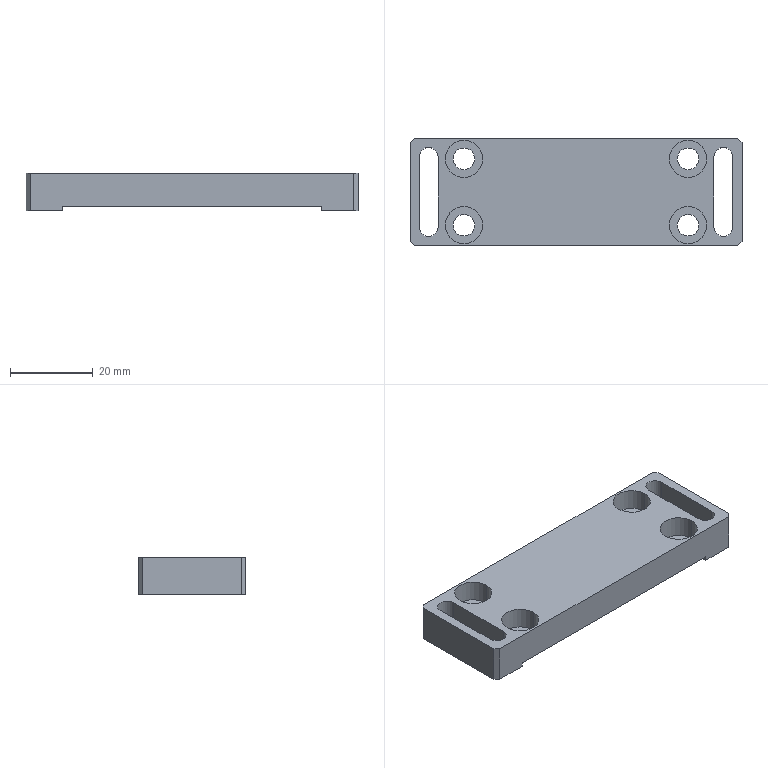Part | SolidWorks | features ICE 4, Chamfer 1, Extrusion 1, MirrorPattern 1 | 1 solid | 42 faces | box 80 x 26 x 9 mm | volume 13853 mm3 | plane 22 | cylinder 20 | commonest cylinder face diameters 5.2 x8 9 x8 4.5 x4
STEP:
#1=CARTESIAN_POINT('',(22.5,-8.,3.8));
#2=VERTEX_POINT('',#1);
#3=CARTESIAN_POINT('',(31.5,-8.,3.8));
#4=VERTEX_POINT('',#3);
#5=CARTESIAN_POINT('',(27.,-8.,3.8));
#6=DIRECTION('',(0.,0.,1.));
#7=DIRECTION('',(1.,0.,0.));
#8=AXIS2_PLACEMENT_3D('',#5,#6,#7);
#9=CIRCLE('',#8,4.5);
#10=EDGE_CURVE('',#2,#4,#9,.T.);
#11=ORIENTED_EDGE('',*,*,#10,.F.);
#12=CARTESIAN_POINT('',(22.5,-8.,9.));
#13=VERTEX_POINT('',#12);
#14=CARTESIAN_POINT('',(22.5,-8.,3.8));
#15=DIRECTION('',(0.,0.,1.));
#16=VECTOR('',#15,1000.);
#17=LINE('',#14,#16);
#18=EDGE_CURVE('',#2,#13,#17,.T.);
#19=ORIENTED_EDGE('',*,*,#18,.T.);
#20=CARTESIAN_POINT('',(31.5,-8.,9.));
#21=VERTEX_POINT('',#20);
#22=CARTESIAN_POINT('',(27.,-8.,9.));
#23=DIRECTION('',(0.,0.,1.));
#24=DIRECTION('',(1.,0.,0.));
#25=AXIS2_PLACEMENT_3D('',#22,#23,#24);
#26=CIRCLE('',#25,4.5);
#27=EDGE_CURVE('',#13,#21,#26,.T.);
#28=ORIENTED_EDGE('',*,*,#27,.T.);
#29=CARTESIAN_POINT('',(31.5,-8.,3.8));
#30=DIRECTION('',(0.,0.,1.));
#31=VECTOR('',#30,1000.);
#32=LINE('',#29,#31);
#33=EDGE_CURVE('',#4,#21,#32,.T.);
#34=ORIENTED_EDGE('',*,*,#33,.F.);
#35=EDGE_LOOP('',(#11,#19,#28,#34));
#36=FACE_OUTER_BOUND('',#35,.T.);
#37=CARTESIAN_POINT('',(27.,-8.,3.8));
#38=DIRECTION('',(0.,0.,1.));
#39=DIRECTION('',(1.,0.,0.));
#40=AXIS2_PLACEMENT_3D('',#37,#38,#39);
#41=CYLINDRICAL_SURFACE('',#40,4.5);
#42=ADVANCED_FACE('',(#36),#41,.F.);
#43=CARTESIAN_POINT('',(22.5,8.,3.8));
#44=VERTEX_POINT('',#43);
#45=CARTESIAN_POINT('',(31.5,8.,3.8));
#46=VERTEX_POINT('',#45);
#47=CARTESIAN_POINT('',(27.,8.,3.8));
#48=DIRECTION('',(0.,0.,1.));
#49=DIRECTION('',(1.,0.,0.));
#50=AXIS2_PLACEMENT_3D('',#47,#48,#49);
#51=CIRCLE('',#50,4.5);
#52=EDGE_CURVE('',#44,#46,#51,.T.);
#53=ORIENTED_EDGE('',*,*,#52,.F.);
#54=CARTESIAN_POINT('',(22.5,8.,9.));
#55=VERTEX_POINT('',#54);
#56=CARTESIAN_POINT('',(22.5,8.,3.8));
#57=DIRECTION('',(0.,0.,1.));
#58=VECTOR('',#57,1000.);
#59=LINE('',#56,#58);
#60=EDGE_CURVE('',#44,#55,#59,.T.);
#61=ORIENTED_EDGE('',*,*,#60,.T.);
#62=CARTESIAN_POINT('',(31.5,8.,9.));
#63=VERTEX_POINT('',#62);
#64=CARTESIAN_POINT('',(27.,8.,9.));
#65=DIRECTION('',(0.,0.,1.));
#66=DIRECTION('',(1.,0.,0.));
#67=AXIS2_PLACEMENT_3D('',#64,#65,#66);
#68=CIRCLE('',#67,4.5);
#69=EDGE_CURVE('',#55,#63,#68,.T.);
#70=ORIENTED_EDGE('',*,*,#69,.T.);
#71=CARTESIAN_POINT('',(31.5,8.,3.8));
#72=DIRECTION('',(0.,0.,1.));
#73=VECTOR('',#72,1000.);
#74=LINE('',#71,#73);
#75=EDGE_CURVE('',#46,#63,#74,.T.);
#76=ORIENTED_EDGE('',*,*,#75,.F.);
#77=EDGE_LOOP('',(#53,#61,#70,#76));
#78=FACE_OUTER_BOUND('',#77,.T.);
#79=CARTESIAN_POINT('',(27.,8.,3.8));
#80=DIRECTION('',(0.,0.,1.));
#81=DIRECTION('',(1.,0.,0.));
#82=AXIS2_PLACEMENT_3D('',#79,#80,#81);
#83=CYLINDRICAL_SURFACE('',#82,4.5);
#84=ADVANCED_FACE('',(#78),#83,.F.);
#85=CARTESIAN_POINT('',(-31.5,8.,3.8));
#86=VERTEX_POINT('',#85);
#87=CARTESIAN_POINT('',(-22.5,8.,3.8));
#88=VERTEX_POINT('',#87);
#89=CARTESIAN_POINT('',(-27.,8.,3.8));
#90=DIRECTION('',(0.,0.,1.));
#91=DIRECTION('',(1.,0.,0.));
#92=AXIS2_PLACEMENT_3D('',#89,#90,#91);
#93=CIRCLE('',#92,4.5);
#94=EDGE_CURVE('',#86,#88,#93,.T.);
#95=ORIENTED_EDGE('',*,*,#94,.F.);
#96=CARTESIAN_POINT('',(-31.5,8.,9.));
#97=VERTEX_POINT('',#96);
#98=CARTESIAN_POINT('',(-31.5,8.,3.8));
#99=DIRECTION('',(0.,0.,1.));
#100=VECTOR('',#99,1000.);
#101=LINE('',#98,#100);
#102=EDGE_CURVE('',#86,#97,#101,.T.);
#103=ORIENTED_EDGE('',*,*,#102,.T.);
#104=CARTESIAN_POINT('',(-22.5,8.,9.));
#105=VERTEX_POINT('',#104);
#106=CARTESIAN_POINT('',(-27.,8.,9.));
#107=DIRECTION('',(0.,0.,1.));
#108=DIRECTION('',(1.,0.,0.));
#109=AXIS2_PLACEMENT_3D('',#106,#107,#108);
#110=CIRCLE('',#109,4.5);
#111=EDGE_CURVE('',#97,#105,#110,.T.);
#112=ORIENTED_EDGE('',*,*,#111,.T.);
#113=CARTESIAN_POINT('',(-22.5,8.,3.8));
#114=DIRECTION('',(0.,0.,1.));
#115=VECTOR('',#114,1000.);
#116=LINE('',#113,#115);
#117=EDGE_CURVE('',#88,#105,#116,.T.);
#118=ORIENTED_EDGE('',*,*,#117,.F.);
#119=EDGE_LOOP('',(#95,#103,#112,#118));
#120=FACE_OUTER_BOUND('',#119,.T.);
#121=CARTESIAN_POINT('',(-27.,8.,3.8));
#122=DIRECTION('',(0.,0.,1.));
#123=DIRECTION('',(1.,0.,0.));
#124=AXIS2_PLACEMENT_3D('',#121,#122,#123);
#125=CYLINDRICAL_SURFACE('',#124,4.5);
#126=ADVANCED_FACE('',(#120),#125,.F.);
#127=CARTESIAN_POINT('',(-31.5,-8.,3.8));
#128=VERTEX_POINT('',#127);
#129=CARTESIAN_POINT('',(-22.5,-8.,3.8));
#130=VERTEX_POINT('',#129);
#131=CARTESIAN_POINT('',(-27.,-8.,3.8));
#132=DIRECTION('',(0.,0.,1.));
#133=DIRECTION('',(1.,0.,0.));
#134=AXIS2_PLACEMENT_3D('',#131,#132,#133);
#135=CIRCLE('',#134,4.5);
#136=EDGE_CURVE('',#128,#130,#135,.T.);
#137=ORIENTED_EDGE('',*,*,#136,.F.);
#138=CARTESIAN_POINT('',(-31.5,-8.,9.));
#139=VERTEX_POINT('',#138);
#140=CARTESIAN_POINT('',(-31.5,-8.,3.8));
#141=DIRECTION('',(0.,0.,1.));
#142=VECTOR('',#141,1000.);
#143=LINE('',#140,#142);
#144=EDGE_CURVE('',#128,#139,#143,.T.);
#145=ORIENTED_EDGE('',*,*,#144,.T.);
#146=CARTESIAN_POINT('',(-22.5,-8.,9.));
#147=VERTEX_POINT('',#146);
#148=CARTESIAN_POINT('',(-27.,-8.,9.));
#149=DIRECTION('',(0.,0.,1.));
#150=DIRECTION('',(1.,0.,0.));
#151=AXIS2_PLACEMENT_3D('',#148,#149,#150);
#152=CIRCLE('',#151,4.5);
#153=EDGE_CURVE('',#139,#147,#152,.T.);
#154=ORIENTED_EDGE('',*,*,#153,.T.);
#155=CARTESIAN_POINT('',(-22.5,-8.,3.8));
#156=DIRECTION('',(0.,0.,1.));
#157=VECTOR('',#156,1000.);
#158=LINE('',#155,#157);
#159=EDGE_CURVE('',#130,#147,#158,.T.);
#160=ORIENTED_EDGE('',*,*,#159,.F.);
#161=EDGE_LOOP('',(#137,#145,#154,#160));
#162=FACE_OUTER_BOUND('',#161,.T.);
#163=CARTESIAN_POINT('',(-27.,-8.,3.8));
#164=DIRECTION('',(0.,0.,1.));
#165=DIRECTION('',(1.,0.,0.));
#166=AXIS2_PLACEMENT_3D('',#163,#164,#165);
#167=CYLINDRICAL_SURFACE('',#166,4.5);
#168=ADVANCED_FACE('',(#162),#167,.F.);
#169=CARTESIAN_POINT('',(-29.6,-8.,1.));
#170=VERTEX_POINT('',#169);
#171=CARTESIAN_POINT('',(-24.4,-8.,1.));
#172=VERTEX_POINT('',#171);
#173=CARTESIAN_POINT('',(-27.,-8.,1.));
#174=DIRECTION('',(0.,0.,1.));
#175=DIRECTION('',(-1.,0.,0.));
#176=AXIS2_PLACEMENT_3D('',#173,#174,#175);
#177=CIRCLE('',#176,2.6);
#178=EDGE_CURVE('',#170,#172,#177,.T.);
#179=ORIENTED_EDGE('',*,*,#178,.F.);
#180=CARTESIAN_POINT('',(-29.6,-8.,3.8));
#181=VERTEX_POINT('',#180);
#182=CARTESIAN_POINT('',(-29.6,-8.,-0.001));
#183=DIRECTION('',(0.,0.,1.));
#184=VECTOR('',#183,1000.);
#185=LINE('',#182,#184);
#186=EDGE_CURVE('',#170,#181,#185,.T.);
#187=ORIENTED_EDGE('',*,*,#186,.T.);
#188=CARTESIAN_POINT('',(-24.4,-8.,3.8));
#189=VERTEX_POINT('',#188);
#190=CARTESIAN_POINT('',(-27.,-8.,3.8));
#191=DIRECTION('',(0.,0.,-1.));
#192=DIRECTION('',(1.,0.,0.));
#193=AXIS2_PLACEMENT_3D('',#190,#191,#192);
#194=CIRCLE('',#193,2.6);
#195=EDGE_CURVE('',#189,#181,#194,.T.);
#196=ORIENTED_EDGE('',*,*,#195,.F.);
#197=CARTESIAN_POINT('',(-24.4,-8.,-0.001));
#198=DIRECTION('',(0.,0.,1.));
#199=VECTOR('',#198,1000.);
#200=LINE('',#197,#199);
#201=EDGE_CURVE('',#172,#189,#200,.T.);
#202=ORIENTED_EDGE('',*,*,#201,.F.);
#203=EDGE_LOOP('',(#179,#187,#196,#202));
#204=FACE_OUTER_BOUND('',#203,.T.);
#205=CARTESIAN_POINT('',(-27.,-8.,-0.001));
#206=DIRECTION('',(0.,0.,1.));
#207=DIRECTION('',(1.,0.,0.));
#208=AXIS2_PLACEMENT_3D('',#205,#206,#207);
#209=CYLINDRICAL_SURFACE('',#208,2.6);
#210=ADVANCED_FACE('',(#204),#209,.F.);
#211=CARTESIAN_POINT('',(-29.6,8.,1.));
#212=VERTEX_POINT('',#211);
#213=CARTESIAN_POINT('',(-24.4,8.,1.));
#214=VERTEX_POINT('',#213);
#215=CARTESIAN_POINT('',(-27.,8.,1.));
#216=DIRECTION('',(0.,0.,1.));
#217=DIRECTION('',(-1.,0.,0.));
#218=AXIS2_PLACEMENT_3D('',#215,#216,#217);
#219=CIRCLE('',#218,2.6);
#220=EDGE_CURVE('',#212,#214,#219,.T.);
#221=ORIENTED_EDGE('',*,*,#220,.F.);
#222=CARTESIAN_POINT('',(-29.6,8.,3.8));
#223=VERTEX_POINT('',#222);
#224=CARTESIAN_POINT('',(-29.6,8.,-0.001));
#225=DIRECTION('',(0.,0.,1.));
#226=VECTOR('',#225,1000.);
#227=LINE('',#224,#226);
#228=EDGE_CURVE('',#212,#223,#227,.T.);
#229=ORIENTED_EDGE('',*,*,#228,.T.);
#230=CARTESIAN_POINT('',(-24.4,8.,3.8));
#231=VERTEX_POINT('',#230);
#232=CARTESIAN_POINT('',(-27.,8.,3.8));
#233=DIRECTION('',(0.,0.,-1.));
#234=DIRECTION('',(1.,0.,0.));
#235=AXIS2_PLACEMENT_3D('',#232,#233,#234);
#236=CIRCLE('',#235,2.6);
#237=EDGE_CURVE('',#231,#223,#236,.T.);
#238=ORIENTED_EDGE('',*,*,#237,.F.);
#239=CARTESIAN_POINT('',(-24.4,8.,-0.001));
#240=DIRECTION('',(0.,0.,1.));
#241=VECTOR('',#240,1000.);
#242=LINE('',#239,#241);
#243=EDGE_CURVE('',#214,#231,#242,.T.);
#244=ORIENTED_EDGE('',*,*,#243,.F.);
#245=EDGE_LOOP('',(#221,#229,#238,#244));
#246=FACE_OUTER_BOUND('',#245,.T.);
#247=CARTESIAN_POINT('',(-27.,8.,-0.001));
#248=DIRECTION('',(0.,0.,1.));
#249=DIRECTION('',(1.,0.,0.));
#250=AXIS2_PLACEMENT_3D('',#247,#248,#249);
#251=CYLINDRICAL_SURFACE('',#250,2.6);
#252=ADVANCED_FACE('',(#246),#251,.F.);
#253=CARTESIAN_POINT('',(24.4,8.,1.));
#254=VERTEX_POINT('',#253);
#255=CARTESIAN_POINT('',(29.6,8.,1.));
#256=VERTEX_POINT('',#255);
#257=CARTESIAN_POINT('',(27.,8.,1.));
#258=DIRECTION('',(0.,0.,1.));
#259=DIRECTION('',(-1.,0.,0.));
#260=AXIS2_PLACEMENT_3D('',#257,#258,#259);
#261=CIRCLE('',#260,2.6);
#262=EDGE_CURVE('',#254,#256,#261,.T.);
#263=ORIENTED_EDGE('',*,*,#262,.F.);
#264=CARTESIAN_POINT('',(24.4,8.,3.8));
#265=VERTEX_POINT('',#264);
#266=CARTESIAN_POINT('',(24.4,8.,-0.001));
#267=DIRECTION('',(0.,0.,1.));
#268=VECTOR('',#267,1000.);
#269=LINE('',#266,#268);
#270=EDGE_CURVE('',#254,#265,#269,.T.);
#271=ORIENTED_EDGE('',*,*,#270,.T.);
#272=CARTESIAN_POINT('',(29.6,8.,3.8));
#273=VERTEX_POINT('',#272);
#274=CARTESIAN_POINT('',(27.,8.,3.8));
#275=DIRECTION('',(0.,0.,-1.));
#276=DIRECTION('',(1.,0.,0.));
#277=AXIS2_PLACEMENT_3D('',#274,#275,#276);
#278=CIRCLE('',#277,2.6);
#279=EDGE_CURVE('',#273,#265,#278,.T.);
#280=ORIENTED_EDGE('',*,*,#279,.F.);
#281=CARTESIAN_POINT('',(29.6,8.,-0.001));
#282=DIRECTION('',(0.,0.,1.));
#283=VECTOR('',#282,1000.);
#284=LINE('',#281,#283);
#285=EDGE_CURVE('',#256,#273,#284,.T.);
#286=ORIENTED_EDGE('',*,*,#285,.F.);
#287=EDGE_LOOP('',(#263,#271,#280,#286));
#288=FACE_OUTER_BOUND('',#287,.T.);
#289=CARTESIAN_POINT('',(27.,8.,-0.001));
#290=DIRECTION('',(0.,0.,1.));
#291=DIRECTION('',(1.,0.,0.));
#292=AXIS2_PLACEMENT_3D('',#289,#290,#291);
#293=CYLINDRICAL_SURFACE('',#292,2.6);
#294=ADVANCED_FACE('',(#288),#293,.F.);
#295=CARTESIAN_POINT('',(24.4,-8.,1.));
#296=VERTEX_POINT('',#295);
#297=CARTESIAN_POINT('',(29.6,-8.,1.));
#298=VERTEX_POINT('',#297);
#299=CARTESIAN_POINT('',(27.,-8.,1.));
#300=DIRECTION('',(0.,0.,1.));
#301=DIRECTION('',(-1.,0.,0.));
#302=AXIS2_PLACEMENT_3D('',#299,#300,#301);
#303=CIRCLE('',#302,2.6);
#304=EDGE_CURVE('',#296,#298,#303,.T.);
#305=ORIENTED_EDGE('',*,*,#304,.F.);
#306=CARTESIAN_POINT('',(24.4,-8.,3.8));
#307=VERTEX_POINT('',#306);
#308=CARTESIAN_POINT('',(24.4,-8.,-0.001));
#309=DIRECTION('',(0.,0.,1.));
#310=VECTOR('',#309,1000.);
#311=LINE('',#308,#310);
#312=EDGE_CURVE('',#296,#307,#311,.T.);
#313=ORIENTED_EDGE('',*,*,#312,.T.);
#314=CARTESIAN_POINT('',(29.6,-8.,3.8));
#315=VERTEX_POINT('',#314);
#316=CARTESIAN_POINT('',(27.,-8.,3.8));
#317=DIRECTION('',(0.,0.,-1.));
#318=DIRECTION('',(1.,0.,0.));
#319=AXIS2_PLACEMENT_3D('',#316,#317,#318);
#320=CIRCLE('',#319,2.6);
#321=EDGE_CURVE('',#315,#307,#320,.T.);
#322=ORIENTED_EDGE('',*,*,#321,.F.);
#323=CARTESIAN_POINT('',(29.6,-8.,-0.001));
#324=DIRECTION('',(0.,0.,1.));
#325=VECTOR('',#324,1000.);
#326=LINE('',#323,#325);
#327=EDGE_CURVE('',#298,#315,#326,.T.);
#328=ORIENTED_EDGE('',*,*,#327,.F.);
#329=EDGE_LOOP('',(#305,#313,#322,#328));
#330=FACE_OUTER_BOUND('',#329,.T.);
#331=CARTESIAN_POINT('',(27.,-8.,-0.001));
#332=DIRECTION('',(0.,0.,1.));
#333=DIRECTION('',(1.,0.,0.));
#334=AXIS2_PLACEMENT_3D('',#331,#332,#333);
#335=CYLINDRICAL_SURFACE('',#334,2.6);
#336=ADVANCED_FACE('',(#330),#335,.F.);
#337=CARTESIAN_POINT('',(-33.25,8.5,0.));
#338=VERTEX_POINT('',#337);
#339=CARTESIAN_POINT('',(-37.75,8.5,0.));
#340=VERTEX_POINT('',#339);
#341=CARTESIAN_POINT('',(-35.5,8.5,0.));
#342=DIRECTION('',(0.,0.,1.));
#343=DIRECTION('',(1.,0.,0.));
#344=AXIS2_PLACEMENT_3D('',#341,#342,#343);
#345=CIRCLE('',#344,2.25);
#346=EDGE_CURVE('',#338,#340,#345,.T.);
#347=ORIENTED_EDGE('',*,*,#346,.T.);
#348=CARTESIAN_POINT('',(-37.75,-8.5,0.));
#349=VERTEX_POINT('',#348);
#350=CARTESIAN_POINT('',(-37.75,8.5,0.));
#351=DIRECTION('',(0.,-1.,0.));
#352=VECTOR('',#351,1000.);
#353=LINE('',#350,#352);
#354=EDGE_CURVE('',#340,#349,#353,.T.);
#355=ORIENTED_EDGE('',*,*,#354,.T.);
#356=CARTESIAN_POINT('',(-33.25,-8.5,0.));
#357=VERTEX_POINT('',#356);
#358=CARTESIAN_POINT('',(-35.5,-8.5,0.));
#359=DIRECTION('',(0.,0.,1.));
#360=DIRECTION('',(1.,0.,0.));
#361=AXIS2_PLACEMENT_3D('',#358,#359,#360);
#362=CIRCLE('',#361,2.25);
#363=EDGE_CURVE('',#349,#357,#362,.T.);
#364=ORIENTED_EDGE('',*,*,#363,.T.);
#365=CARTESIAN_POINT('',(-33.25,8.5,0.));
#366=DIRECTION('',(0.,1.,0.));
#367=VECTOR('',#366,1000.);
#368=LINE('',#365,#367);
#369=EDGE_CURVE('',#357,#338,#368,.T.);
#370=ORIENTED_EDGE('',*,*,#369,.T.);
#371=EDGE_LOOP('',(#347,#355,#364,#370));
#372=FACE_BOUND('',#371,.T.);
#373=CARTESIAN_POINT('',(-39.,-13.,0.));
#374=VERTEX_POINT('',#373);
#375=CARTESIAN_POINT('',(-31.25,-13.,0.));
#376=VERTEX_POINT('',#375);
#377=CARTESIAN_POINT('',(-40.,-13.,0.));
#378=DIRECTION('',(1.,0.,0.));
#379=VECTOR('',#378,1000.);
#380=LINE('',#377,#379);
#381=EDGE_CURVE('',#374,#376,#380,.T.);
#382=ORIENTED_EDGE('',*,*,#381,.F.);
#383=CARTESIAN_POINT('',(-40.,-12.,0.));
#384=VERTEX_POINT('',#383);
#385=CARTESIAN_POINT('',(-39.,-13.,0.));
#386=DIRECTION('',(-0.7071,0.7071,0.));
#387=VECTOR('',#386,1000.);
#388=LINE('',#385,#387);
#389=EDGE_CURVE('',#374,#384,#388,.T.);
#390=ORIENTED_EDGE('',*,*,#389,.T.);
#391=CARTESIAN_POINT('',(-40.,12.,0.));
#392=VERTEX_POINT('',#391);
#393=CARTESIAN_POINT('',(-40.,13.,0.));
#394=DIRECTION('',(0.,-1.,0.));
#395=VECTOR('',#394,1000.);
#396=LINE('',#393,#395);
#397=EDGE_CURVE('',#392,#384,#396,.T.);
#398=ORIENTED_EDGE('',*,*,#397,.F.);
#399=CARTESIAN_POINT('',(-39.,13.,0.));
#400=VERTEX_POINT('',#399);
#401=CARTESIAN_POINT('',(-40.,12.,0.));
#402=DIRECTION('',(0.7071,0.7071,0.));
#403=VECTOR('',#402,1000.);
#404=LINE('',#401,#403);
#405=EDGE_CURVE('',#392,#400,#404,.T.);
#406=ORIENTED_EDGE('',*,*,#405,.T.);
#407=CARTESIAN_POINT('',(-31.25,13.,0.));
#408=VERTEX_POINT('',#407);
#409=CARTESIAN_POINT('',(-40.,13.,0.));
#410=DIRECTION('',(-1.,0.,0.));
#411=VECTOR('',#410,1000.);
#412=LINE('',#409,#411);
#413=EDGE_CURVE('',#408,#400,#412,.T.);
#414=ORIENTED_EDGE('',*,*,#413,.F.);
#415=CARTESIAN_POINT('',(-31.25,13.,0.));
#416=DIRECTION('',(0.,1.,0.));
#417=VECTOR('',#416,1000.);
#418=LINE('',#415,#417);
#419=EDGE_CURVE('',#376,#408,#418,.T.);
#420=ORIENTED_EDGE('',*,*,#419,.F.);
#421=EDGE_LOOP('',(#382,#390,#398,#406,#414,#420));
#422=FACE_OUTER_BOUND('',#421,.T.);
#423=CARTESIAN_POINT('',(40.,-13.,0.));
#424=DIRECTION('',(0.,0.,1.));
#425=DIRECTION('',(1.,0.,0.));
#426=AXIS2_PLACEMENT_3D('',#423,#424,#425);
#427=PLANE('',#426);
#428=ADVANCED_FACE('',(#372,#422),#427,.F.);
#429=ORIENTED_EDGE('',*,*,#312,.F.);
#430=CARTESIAN_POINT('',(27.,-8.,1.));
#431=DIRECTION('',(0.,0.,1.));
#432=DIRECTION('',(-1.,0.,0.));
#433=AXIS2_PLACEMENT_3D('',#430,#431,#432);
#434=CIRCLE('',#433,2.6);
#435=EDGE_CURVE('',#298,#296,#434,.T.);
#436=ORIENTED_EDGE('',*,*,#435,.F.);
#437=ORIENTED_EDGE('',*,*,#327,.T.);
#438=CARTESIAN_POINT('',(27.,-8.,3.8));
#439=DIRECTION('',(0.,0.,-1.));
#440=DIRECTION('',(1.,0.,0.));
#441=AXIS2_PLACEMENT_3D('',#438,#439,#440);
#442=CIRCLE('',#441,2.6);
#443=EDGE_CURVE('',#307,#315,#442,.T.);
#444=ORIENTED_EDGE('',*,*,#443,.F.);
#445=EDGE_LOOP('',(#429,#436,#437,#444));
#446=FACE_OUTER_BOUND('',#445,.T.);
#447=CARTESIAN_POINT('',(27.,-8.,-0.001));
#448=DIRECTION('',(0.,0.,1.));
#449=DIRECTION('',(1.,0.,0.));
#450=AXIS2_PLACEMENT_3D('',#447,#448,#449);
#451=CYLINDRICAL_SURFACE('',#450,2.6);
#452=ADVANCED_FACE('',(#446),#451,.F.);
#453=ORIENTED_EDGE('',*,*,#270,.F.);
#454=CARTESIAN_POINT('',(27.,8.,1.));
#455=DIRECTION('',(0.,0.,1.));
#456=DIRECTION('',(-1.,0.,0.));
#457=AXIS2_PLACEMENT_3D('',#454,#455,#456);
#458=CIRCLE('',#457,2.6);
#459=EDGE_CURVE('',#256,#254,#458,.T.);
#460=ORIENTED_EDGE('',*,*,#459,.F.);
#461=ORIENTED_EDGE('',*,*,#285,.T.);
#462=CARTESIAN_POINT('',(27.,8.,3.8));
#463=DIRECTION('',(0.,0.,-1.));
#464=DIRECTION('',(1.,0.,0.));
#465=AXIS2_PLACEMENT_3D('',#462,#463,#464);
#466=CIRCLE('',#465,2.6);
#467=EDGE_CURVE('',#265,#273,#466,.T.);
#468=ORIENTED_EDGE('',*,*,#467,.F.);
#469=EDGE_LOOP('',(#453,#460,#461,#468));
#470=FACE_OUTER_BOUND('',#469,.T.);
#471=CARTESIAN_POINT('',(27.,8.,-0.001));
#472=DIRECTION('',(0.,0.,1.));
#473=DIRECTION('',(1.,0.,0.));
#474=AXIS2_PLACEMENT_3D('',#471,#472,#473);
#475=CYLINDRICAL_SURFACE('',#474,2.6);
#476=ADVANCED_FACE('',(#470),#475,.F.);
#477=ORIENTED_EDGE('',*,*,#228,.F.);
#478=CARTESIAN_POINT('',(-27.,8.,1.));
#479=DIRECTION('',(0.,0.,1.));
#480=DIRECTION('',(-1.,0.,0.));
#481=AXIS2_PLACEMENT_3D('',#478,#479,#480);
#482=CIRCLE('',#481,2.6);
#483=EDGE_CURVE('',#214,#212,#482,.T.);
#484=ORIENTED_EDGE('',*,*,#483,.F.);
#485=ORIENTED_EDGE('',*,*,#243,.T.);
#486=CARTESIAN_POINT('',(-27.,8.,3.8));
#487=DIRECTION('',(0.,0.,-1.));
#488=DIRECTION('',(1.,0.,0.));
#489=AXIS2_PLACEMENT_3D('',#486,#487,#488);
#490=CIRCLE('',#489,2.6);
#491=EDGE_CURVE('',#223,#231,#490,.T.);
#492=ORIENTED_EDGE('',*,*,#491,.F.);
#493=EDGE_LOOP('',(#477,#484,#485,#492));
#494=FACE_OUTER_BOUND('',#493,.T.);
#495=CARTESIAN_POINT('',(-27.,8.,-0.001));
#496=DIRECTION('',(0.,0.,1.));
#497=DIRECTION('',(1.,0.,0.));
#498=AXIS2_PLACEMENT_3D('',#495,#496,#497);
#499=CYLINDRICAL_SURFACE('',#498,2.6);
#500=ADVANCED_FACE('',(#494),#499,.F.);
#501=ORIENTED_EDGE('',*,*,#186,.F.);
#502=CARTESIAN_POINT('',(-27.,-8.,1.));
#503=DIRECTION('',(0.,0.,1.));
#504=DIRECTION('',(-1.,0.,0.));
#505=AXIS2_PLACEMENT_3D('',#502,#503,#504);
#506=CIRCLE('',#505,2.6);
#507=EDGE_CURVE('',#172,#170,#506,.T.);
#508=ORIENTED_EDGE('',*,*,#507,.F.);
#509=ORIENTED_EDGE('',*,*,#201,.T.);
#510=CARTESIAN_POINT('',(-27.,-8.,3.8));
#511=DIRECTION('',(0.,0.,-1.));
#512=DIRECTION('',(1.,0.,0.));
#513=AXIS2_PLACEMENT_3D('',#510,#511,#512);
#514=CIRCLE('',#513,2.6);
#515=EDGE_CURVE('',#181,#189,#514,.T.);
#516=ORIENTED_EDGE('',*,*,#515,.F.);
#517=EDGE_LOOP('',(#501,#508,#509,#516));
#518=FACE_OUTER_BOUND('',#517,.T.);
#519=CARTESIAN_POINT('',(-27.,-8.,-0.001));
#520=DIRECTION('',(0.,0.,1.));
#521=DIRECTION('',(1.,0.,0.));
#522=AXIS2_PLACEMENT_3D('',#519,#520,#521);
#523=CYLINDRICAL_SURFACE('',#522,2.6);
#524=ADVANCED_FACE('',(#518),#523,.F.);
#525=CARTESIAN_POINT('',(40.,-12.,9.));
#526=VERTEX_POINT('',#525);
#527=CARTESIAN_POINT('',(40.,12.,9.));
#528=VERTEX_POINT('',#527);
#529=CARTESIAN_POINT('',(40.,13.,9.));
#530=DIRECTION('',(0.,1.,0.));
#531=VECTOR('',#530,1000.);
#532=LINE('',#529,#531);
#533=EDGE_CURVE('',#526,#528,#532,.T.);
#534=ORIENTED_EDGE('',*,*,#533,.T.);
#535=CARTESIAN_POINT('',(39.,13.,9.));
#536=VERTEX_POINT('',#535);
#537=CARTESIAN_POINT('',(52.5,-0.5,9.));
#538=DIRECTION('',(-0.7071,0.7071,0.));
#539=VECTOR('',#538,1000.);
#540=LINE('',#537,#539);
#541=EDGE_CURVE('',#528,#536,#540,.T.);
#542=ORIENTED_EDGE('',*,*,#541,.T.);
#543=CARTESIAN_POINT('',(-39.,13.,9.));
#544=VERTEX_POINT('',#543);
#545=CARTESIAN_POINT('',(-40.,13.,9.));
#546=DIRECTION('',(-1.,0.,0.));
#547=VECTOR('',#546,1000.);
#548=LINE('',#545,#547);
#549=EDGE_CURVE('',#536,#544,#548,.T.);
#550=ORIENTED_EDGE('',*,*,#549,.T.);
#551=CARTESIAN_POINT('',(-40.,12.,9.));
#552=VERTEX_POINT('',#551);
#553=CARTESIAN_POINT('',(-12.5,39.5,9.));
#554=DIRECTION('',(-0.7071,-0.7071,0.));
#555=VECTOR('',#554,1000.);
#556=LINE('',#553,#555);
#557=EDGE_CURVE('',#544,#552,#556,.T.);
#558=ORIENTED_EDGE('',*,*,#557,.T.);
#559=CARTESIAN_POINT('',(-40.,-12.,9.));
#560=VERTEX_POINT('',#559);
#561=CARTESIAN_POINT('',(-40.,13.,9.));
#562=DIRECTION('',(0.,-1.,0.));
#563=VECTOR('',#562,1000.);
#564=LINE('',#561,#563);
#565=EDGE_CURVE('',#552,#560,#564,.T.);
#566=ORIENTED_EDGE('',*,*,#565,.T.);
#567=CARTESIAN_POINT('',(-39.,-13.,9.));
#568=VERTEX_POINT('',#567);
#569=CARTESIAN_POINT('',(0.5,-52.5,9.));
#570=DIRECTION('',(0.7071,-0.7071,0.));
#571=VECTOR('',#570,1000.);
#572=LINE('',#569,#571);
#573=EDGE_CURVE('',#560,#568,#572,.T.);
#574=ORIENTED_EDGE('',*,*,#573,.T.);
#575=CARTESIAN_POINT('',(39.,-13.,9.));
#576=VERTEX_POINT('',#575);
#577=CARTESIAN_POINT('',(-40.,-13.,9.));
#578=DIRECTION('',(1.,0.,0.));
#579=VECTOR('',#578,1000.);
#580=LINE('',#577,#579);
#581=EDGE_CURVE('',#568,#576,#580,.T.);
#582=ORIENTED_EDGE('',*,*,#581,.T.);
#583=CARTESIAN_POINT('',(39.5,-12.5,9.));
#584=DIRECTION('',(0.7071,0.7071,0.));
#585=VECTOR('',#584,1000.);
#586=LINE('',#583,#585);
#587=EDGE_CURVE('',#576,#526,#586,.T.);
#588=ORIENTED_EDGE('',*,*,#587,.T.);
#589=EDGE_LOOP('',(#534,#542,#550,#558,#566,#574,#582,#588));
#590=FACE_OUTER_BOUND('',#589,.T.);
#591=CARTESIAN_POINT('',(-27.,-8.,9.));
#592=DIRECTION('',(0.,0.,1.));
#593=DIRECTION('',(1.,0.,0.));
#594=AXIS2_PLACEMENT_3D('',#591,#592,#593);
#595=CIRCLE('',#594,4.5);
#596=EDGE_CURVE('',#147,#139,#595,.T.);
#597=ORIENTED_EDGE('',*,*,#596,.F.);
#598=ORIENTED_EDGE('',*,*,#153,.F.);
#599=EDGE_LOOP('',(#597,#598));
#600=FACE_BOUND('',#599,.T.);
#601=CARTESIAN_POINT('',(-27.,8.,9.));
#602=DIRECTION('',(0.,0.,1.));
#603=DIRECTION('',(1.,0.,0.));
#604=AXIS2_PLACEMENT_3D('',#601,#602,#603);
#605=CIRCLE('',#604,4.5);
#606=EDGE_CURVE('',#105,#97,#605,.T.);
#607=ORIENTED_EDGE('',*,*,#606,.F.);
#608=ORIENTED_EDGE('',*,*,#111,.F.);
#609=EDGE_LOOP('',(#607,#608));
#610=FACE_BOUND('',#609,.T.);
#611=CARTESIAN_POINT('',(27.,8.,9.));
#612=DIRECTION('',(0.,0.,1.));
#613=DIRECTION('',(1.,0.,0.));
#614=AXIS2_PLACEMENT_3D('',#611,#612,#613);
#615=CIRCLE('',#614,4.5);
#616=EDGE_CURVE('',#63,#55,#615,.T.);
#617=ORIENTED_EDGE('',*,*,#616,.F.);
#618=ORIENTED_EDGE('',*,*,#69,.F.);
#619=EDGE_LOOP('',(#617,#618));
#620=FACE_BOUND('',#619,.T.);
#621=CARTESIAN_POINT('',(27.,-8.,9.));
#622=DIRECTION('',(0.,0.,1.));
#623=DIRECTION('',(1.,0.,0.));
#624=AXIS2_PLACEMENT_3D('',#621,#622,#623);
#625=CIRCLE('',#624,4.5);
#626=EDGE_CURVE('',#21,#13,#625,.T.);
#627=ORIENTED_EDGE('',*,*,#626,.F.);
#628=ORIENTED_EDGE('',*,*,#27,.F.);
#629=EDGE_LOOP('',(#627,#628));
#630=FACE_BOUND('',#629,.T.);
#631=CARTESIAN_POINT('',(33.25,8.5,9.));
#632=VERTEX_POINT('',#631);
#633=CARTESIAN_POINT('',(37.75,8.5,9.));
#634=VERTEX_POINT('',#633);
#635=CARTESIAN_POINT('',(35.5,8.5,9.));
#636=DIRECTION('',(0.,0.,-1.));
#637=DIRECTION('',(1.,0.,0.));
#638=AXIS2_PLACEMENT_3D('',#635,#636,#637);
#639=CIRCLE('',#638,2.25);
#640=EDGE_CURVE('',#632,#634,#639,.T.);
#641=ORIENTED_EDGE('',*,*,#640,.T.);
#642=CARTESIAN_POINT('',(37.75,-8.5,9.));
#643=VERTEX_POINT('',#642);
#644=CARTESIAN_POINT('',(37.75,8.5,9.));
#645=DIRECTION('',(0.,-1.,0.));
#646=VECTOR('',#645,1000.);
#647=LINE('',#644,#646);
#648=EDGE_CURVE('',#634,#643,#647,.T.);
#649=ORIENTED_EDGE('',*,*,#648,.T.);
#650=CARTESIAN_POINT('',(33.25,-8.5,9.));
#651=VERTEX_POINT('',#650);
#652=CARTESIAN_POINT('',(35.5,-8.5,9.));
#653=DIRECTION('',(0.,0.,-1.));
#654=DIRECTION('',(1.,0.,0.));
#655=AXIS2_PLACEMENT_3D('',#652,#653,#654);
#656=CIRCLE('',#655,2.25);
#657=EDGE_CURVE('',#643,#651,#656,.T.);
#658=ORIENTED_EDGE('',*,*,#657,.T.);
#659=CARTESIAN_POINT('',(33.25,8.5,9.));
#660=DIRECTION('',(0.,1.,0.));
#661=VECTOR('',#660,1000.);
#662=LINE('',#659,#661);
#663=EDGE_CURVE('',#651,#632,#662,.T.);
#664=ORIENTED_EDGE('',*,*,#663,.T.);
#665=EDGE_LOOP('',(#641,#649,#658,#664));
#666=FACE_BOUND('',#665,.T.);
#667=CARTESIAN_POINT('',(-37.75,8.5,9.));
#668=VERTEX_POINT('',#667);
#669=CARTESIAN_POINT('',(-37.75,-8.5,9.));
#670=VERTEX_POINT('',#669);
#671=CARTESIAN_POINT('',(-37.75,8.5,9.));
#672=DIRECTION('',(0.,-1.,0.));
#673=VECTOR('',#672,1000.);
#674=LINE('',#671,#673);
#675=EDGE_CURVE('',#668,#670,#674,.T.);
#676=ORIENTED_EDGE('',*,*,#675,.F.);
#677=CARTESIAN_POINT('',(-33.25,8.5,9.));
#678=VERTEX_POINT('',#677);
#679=CARTESIAN_POINT('',(-35.5,8.5,9.));
#680=DIRECTION('',(0.,0.,1.));
#681=DIRECTION('',(1.,0.,0.));
#682=AXIS2_PLACEMENT_3D('',#679,#680,#681);
#683=CIRCLE('',#682,2.25);
#684=EDGE_CURVE('',#678,#668,#683,.T.);
#685=ORIENTED_EDGE('',*,*,#684,.F.);
#686=CARTESIAN_POINT('',(-33.25,-8.5,9.));
#687=VERTEX_POINT('',#686);
#688=CARTESIAN_POINT('',(-33.25,8.5,9.));
#689=DIRECTION('',(0.,1.,0.));
#690=VECTOR('',#689,1000.);
#691=LINE('',#688,#690);
#692=EDGE_CURVE('',#687,#678,#691,.T.);
#693=ORIENTED_EDGE('',*,*,#692,.F.);
#694=CARTESIAN_POINT('',(-35.5,-8.5,9.));
#695=DIRECTION('',(0.,0.,1.));
#696=DIRECTION('',(1.,0.,0.));
#697=AXIS2_PLACEMENT_3D('',#694,#695,#696);
#698=CIRCLE('',#697,2.25);
#699=EDGE_CURVE('',#670,#687,#698,.T.);
#700=ORIENTED_EDGE('',*,*,#699,.F.);
#701=EDGE_LOOP('',(#676,#685,#693,#700));
#702=FACE_BOUND('',#701,.T.);
#703=CARTESIAN_POINT('',(40.,-13.,9.));
#704=DIRECTION('',(0.,0.,1.));
#705=DIRECTION('',(1.,0.,0.));
#706=AXIS2_PLACEMENT_3D('',#703,#704,#705);
#707=PLANE('',#706);
#708=ADVANCED_FACE('',(#590,#600,#610,#620,#630,#666,#702),#707,.T.);
#709=CARTESIAN_POINT('',(39.,13.,0.));
#710=VERTEX_POINT('',#709);
#711=CARTESIAN_POINT('',(31.25,13.,0.));
#712=VERTEX_POINT('',#711);
#713=CARTESIAN_POINT('',(-40.,13.,0.));
#714=DIRECTION('',(-1.,0.,0.));
#715=VECTOR('',#714,1000.);
#716=LINE('',#713,#715);
#717=EDGE_CURVE('',#710,#712,#716,.T.);
#718=ORIENTED_EDGE('',*,*,#717,.F.);
#719=CARTESIAN_POINT('',(40.,12.,0.));
#720=VERTEX_POINT('',#719);
#721=CARTESIAN_POINT('',(39.,13.,0.));
#722=DIRECTION('',(0.7071,-0.7071,0.));
#723=VECTOR('',#722,1000.);
#724=LINE('',#721,#723);
#725=EDGE_CURVE('',#710,#720,#724,.T.);
#726=ORIENTED_EDGE('',*,*,#725,.T.);
#727=CARTESIAN_POINT('',(40.,-12.,0.));
#728=VERTEX_POINT('',#727);
#729=CARTESIAN_POINT('',(40.,13.,0.));
#730=DIRECTION('',(0.,1.,0.));
#731=VECTOR('',#730,1000.);
#732=LINE('',#729,#731);
#733=EDGE_CURVE('',#728,#720,#732,.T.);
#734=ORIENTED_EDGE('',*,*,#733,.F.);
#735=CARTESIAN_POINT('',(39.,-13.,0.));
#736=VERTEX_POINT('',#735);
#737=CARTESIAN_POINT('',(40.,-12.,0.));
#738=DIRECTION('',(-0.7071,-0.7071,0.));
#739=VECTOR('',#738,1000.);
#740=LINE('',#737,#739);
#741=EDGE_CURVE('',#728,#736,#740,.T.);
#742=ORIENTED_EDGE('',*,*,#741,.T.);
#743=CARTESIAN_POINT('',(31.25,-13.,0.));
#744=VERTEX_POINT('',#743);
#745=CARTESIAN_POINT('',(-40.,-13.,0.));
#746=DIRECTION('',(1.,0.,0.));
#747=VECTOR('',#746,1000.);
#748=LINE('',#745,#747);
#749=EDGE_CURVE('',#744,#736,#748,.T.);
#750=ORIENTED_EDGE('',*,*,#749,.F.);
#751=CARTESIAN_POINT('',(31.25,13.,0.));
#752=DIRECTION('',(0.,-1.,0.));
#753=VECTOR('',#752,1000.);
#754=LINE('',#751,#753);
#755=EDGE_CURVE('',#712,#744,#754,.T.);
#756=ORIENTED_EDGE('',*,*,#755,.F.);
#757=EDGE_LOOP('',(#718,#726,#734,#742,#750,#756));
#758=FACE_OUTER_BOUND('',#757,.T.);
#759=CARTESIAN_POINT('',(37.75,8.5,0.));
#760=VERTEX_POINT('',#759);
#761=CARTESIAN_POINT('',(37.75,-8.5,0.));
#762=VERTEX_POINT('',#761);
#763=CARTESIAN_POINT('',(37.75,8.5,0.));
#764=DIRECTION('',(0.,-1.,0.));
#765=VECTOR('',#764,1000.);
#766=LINE('',#763,#765);
#767=EDGE_CURVE('',#760,#762,#766,.T.);
#768=ORIENTED_EDGE('',*,*,#767,.F.);
#769=CARTESIAN_POINT('',(33.25,8.5,0.));
#770=VERTEX_POINT('',#769);
#771=CARTESIAN_POINT('',(35.5,8.5,0.));
#772=DIRECTION('',(0.,0.,-1.));
#773=DIRECTION('',(-1.,0.,0.));
#774=AXIS2_PLACEMENT_3D('',#771,#772,#773);
#775=CIRCLE('',#774,2.25);
#776=EDGE_CURVE('',#770,#760,#775,.T.);
#777=ORIENTED_EDGE('',*,*,#776,.F.);
#778=CARTESIAN_POINT('',(33.25,-8.5,0.));
#779=VERTEX_POINT('',#778);
#780=CARTESIAN_POINT('',(33.25,8.5,0.));
#781=DIRECTION('',(0.,1.,0.));
#782=VECTOR('',#781,1000.);
#783=LINE('',#780,#782);
#784=EDGE_CURVE('',#779,#770,#783,.T.);
#785=ORIENTED_EDGE('',*,*,#784,.F.);
#786=CARTESIAN_POINT('',(35.5,-8.5,0.));
#787=DIRECTION('',(0.,0.,-1.));
#788=DIRECTION('',(-1.,0.,0.));
#789=AXIS2_PLACEMENT_3D('',#786,#787,#788);
#790=CIRCLE('',#789,2.25);
#791=EDGE_CURVE('',#762,#779,#790,.T.);
#792=ORIENTED_EDGE('',*,*,#791,.F.);
#793=EDGE_LOOP('',(#768,#777,#785,#792));
#794=FACE_BOUND('',#793,.T.);
#795=CARTESIAN_POINT('',(40.,-13.,0.));
#796=DIRECTION('',(0.,0.,1.));
#797=DIRECTION('',(1.,0.,0.));
#798=AXIS2_PLACEMENT_3D('',#795,#796,#797);
#799=PLANE('',#798);
#800=ADVANCED_FACE('',(#758,#794),#799,.F.);
#801=ORIENTED_EDGE('',*,*,#733,.T.);
#802=CARTESIAN_POINT('',(40.,12.,9.));
#803=DIRECTION('',(0.,0.,1.));
#804=VECTOR('',#803,1000.);
#805=LINE('',#802,#804);
#806=EDGE_CURVE('',#720,#528,#805,.T.);
#807=ORIENTED_EDGE('',*,*,#806,.T.);
#808=ORIENTED_EDGE('',*,*,#533,.F.);
#809=CARTESIAN_POINT('',(40.,-12.,9.));
#810=DIRECTION('',(0.,0.,-1.));
#811=VECTOR('',#810,1000.);
#812=LINE('',#809,#811);
#813=EDGE_CURVE('',#526,#728,#812,.T.);
#814=ORIENTED_EDGE('',*,*,#813,.T.);
#815=EDGE_LOOP('',(#801,#807,#808,#814));
#816=FACE_OUTER_BOUND('',#815,.T.);
#817=CARTESIAN_POINT('',(40.,13.,9.));
#818=DIRECTION('',(-1.,0.,0.));
#819=DIRECTION('',(0.,-1.,0.));
#820=AXIS2_PLACEMENT_3D('',#817,#818,#819);
#821=PLANE('',#820);
#822=ADVANCED_FACE('',(#816),#821,.F.);
#823=ORIENTED_EDGE('',*,*,#549,.F.);
#824=CARTESIAN_POINT('',(39.,13.,9.));
#825=DIRECTION('',(0.,0.,-1.));
#826=VECTOR('',#825,1000.);
#827=LINE('',#824,#826);
#828=EDGE_CURVE('',#536,#710,#827,.T.);
#829=ORIENTED_EDGE('',*,*,#828,.T.);
#830=ORIENTED_EDGE('',*,*,#717,.T.);
#831=CARTESIAN_POINT('',(31.25,13.,1.));
#832=VERTEX_POINT('',#831);
#833=CARTESIAN_POINT('',(31.25,13.,1.));
#834=DIRECTION('',(0.,0.,-1.));
#835=VECTOR('',#834,1000.);
#836=LINE('',#833,#835);
#837=EDGE_CURVE('',#832,#712,#836,.T.);
#838=ORIENTED_EDGE('',*,*,#837,.F.);
#839=CARTESIAN_POINT('',(-31.25,13.,1.));
#840=VERTEX_POINT('',#839);
#841=CARTESIAN_POINT('',(31.25,13.,1.));
#842=DIRECTION('',(1.,0.,0.));
#843=VECTOR('',#842,1000.);
#844=LINE('',#841,#843);
#845=EDGE_CURVE('',#840,#832,#844,.T.);
#846=ORIENTED_EDGE('',*,*,#845,.F.);
#847=CARTESIAN_POINT('',(-31.25,13.,1.));
#848=DIRECTION('',(0.,0.,-1.));
#849=VECTOR('',#848,1000.);
#850=LINE('',#847,#849);
#851=EDGE_CURVE('',#840,#408,#850,.T.);
#852=ORIENTED_EDGE('',*,*,#851,.T.);
#853=ORIENTED_EDGE('',*,*,#413,.T.);
#854=CARTESIAN_POINT('',(-39.,13.,9.));
#855=DIRECTION('',(0.,0.,1.));
#856=VECTOR('',#855,1000.);
#857=LINE('',#854,#856);
#858=EDGE_CURVE('',#400,#544,#857,.T.);
#859=ORIENTED_EDGE('',*,*,#858,.T.);
#860=EDGE_LOOP('',(#823,#829,#830,#838,#846,#852,#853,#859));
#861=FACE_OUTER_BOUND('',#860,.T.);
#862=CARTESIAN_POINT('',(-40.,13.,9.));
#863=DIRECTION('',(0.,-1.,0.));
#864=DIRECTION('',(0.,0.,-1.));
#865=AXIS2_PLACEMENT_3D('',#862,#863,#864);
#866=PLANE('',#865);
#867=ADVANCED_FACE('',(#861),#866,.F.);
#868=ORIENTED_EDGE('',*,*,#397,.T.);
#869=CARTESIAN_POINT('',(-40.,-12.,9.));
#870=DIRECTION('',(0.,0.,1.));
#871=VECTOR('',#870,1000.);
#872=LINE('',#869,#871);
#873=EDGE_CURVE('',#384,#560,#872,.T.);
#874=ORIENTED_EDGE('',*,*,#873,.T.);
#875=ORIENTED_EDGE('',*,*,#565,.F.);
#876=CARTESIAN_POINT('',(-40.,12.,9.));
#877=DIRECTION('',(0.,0.,-1.));
#878=VECTOR('',#877,1000.);
#879=LINE('',#876,#878);
#880=EDGE_CURVE('',#552,#392,#879,.T.);
#881=ORIENTED_EDGE('',*,*,#880,.T.);
#882=EDGE_LOOP('',(#868,#874,#875,#881));
#883=FACE_OUTER_BOUND('',#882,.T.);
#884=CARTESIAN_POINT('',(-40.,13.,9.));
#885=DIRECTION('',(1.,0.,0.));
#886=DIRECTION('',(0.,1.,0.));
#887=AXIS2_PLACEMENT_3D('',#884,#885,#886);
#888=PLANE('',#887);
#889=ADVANCED_FACE('',(#883),#888,.F.);
#890=ORIENTED_EDGE('',*,*,#749,.T.);
#891=CARTESIAN_POINT('',(39.,-13.,9.));
#892=DIRECTION('',(0.,0.,1.));
#893=VECTOR('',#892,1000.);
#894=LINE('',#891,#893);
#895=EDGE_CURVE('',#736,#576,#894,.T.);
#896=ORIENTED_EDGE('',*,*,#895,.T.);
#897=ORIENTED_EDGE('',*,*,#581,.F.);
#898=CARTESIAN_POINT('',(-39.,-13.,9.));
#899=DIRECTION('',(0.,0.,-1.));
#900=VECTOR('',#899,1000.);
#901=LINE('',#898,#900);
#902=EDGE_CURVE('',#568,#374,#901,.T.);
#903=ORIENTED_EDGE('',*,*,#902,.T.);
#904=ORIENTED_EDGE('',*,*,#381,.T.);
#905=CARTESIAN_POINT('',(-31.25,-13.,1.));
#906=VERTEX_POINT('',#905);
#907=CARTESIAN_POINT('',(-31.25,-13.,1.));
#908=DIRECTION('',(0.,0.,-1.));
#909=VECTOR('',#908,1000.);
#910=LINE('',#907,#909);
#911=EDGE_CURVE('',#906,#376,#910,.T.);
#912=ORIENTED_EDGE('',*,*,#911,.F.);
#913=CARTESIAN_POINT('',(31.25,-13.,1.));
#914=VERTEX_POINT('',#913);
#915=CARTESIAN_POINT('',(31.25,-13.,1.));
#916=DIRECTION('',(-1.,0.,0.));
#917=VECTOR('',#916,1000.);
#918=LINE('',#915,#917);
#919=EDGE_CURVE('',#914,#906,#918,.T.);
#920=ORIENTED_EDGE('',*,*,#919,.F.);
#921=CARTESIAN_POINT('',(31.25,-13.,1.));
#922=DIRECTION('',(0.,0.,-1.));
#923=VECTOR('',#922,1000.);
#924=LINE('',#921,#923);
#925=EDGE_CURVE('',#914,#744,#924,.T.);
#926=ORIENTED_EDGE('',*,*,#925,.T.);
#927=EDGE_LOOP('',(#890,#896,#897,#903,#904,#912,#920,#926));
#928=FACE_OUTER_BOUND('',#927,.T.);
#929=CARTESIAN_POINT('',(-40.,-13.,9.));
#930=DIRECTION('',(0.,1.,0.));
#931=DIRECTION('',(0.,0.,1.));
#932=AXIS2_PLACEMENT_3D('',#929,#930,#931);
#933=PLANE('',#932);
#934=ADVANCED_FACE('',(#928),#933,.F.);
#935=CARTESIAN_POINT('',(-27.,-8.,3.8));
#936=DIRECTION('',(0.,0.,1.));
#937=DIRECTION('',(1.,0.,0.));
#938=AXIS2_PLACEMENT_3D('',#935,#936,#937);
#939=CIRCLE('',#938,4.5);
#940=EDGE_CURVE('',#130,#128,#939,.T.);
#941=ORIENTED_EDGE('',*,*,#940,.T.);
#942=ORIENTED_EDGE('',*,*,#136,.T.);
#943=EDGE_LOOP('',(#941,#942));
#944=FACE_OUTER_BOUND('',#943,.T.);
#945=ORIENTED_EDGE('',*,*,#195,.T.);
#946=ORIENTED_EDGE('',*,*,#515,.T.);
#947=EDGE_LOOP('',(#945,#946));
#948=FACE_BOUND('',#947,.T.);
#949=CARTESIAN_POINT('',(-27.,-8.,3.8));
#950=DIRECTION('',(0.,0.,1.));
#951=DIRECTION('',(1.,0.,0.));
#952=AXIS2_PLACEMENT_3D('',#949,#950,#951);
#953=PLANE('',#952);
#954=ADVANCED_FACE('',(#944,#948),#953,.T.);
#955=ORIENTED_EDGE('',*,*,#144,.F.);
#956=ORIENTED_EDGE('',*,*,#940,.F.);
#957=ORIENTED_EDGE('',*,*,#159,.T.);
#958=ORIENTED_EDGE('',*,*,#596,.T.);
#959=EDGE_LOOP('',(#955,#956,#957,#958));
#960=FACE_OUTER_BOUND('',#959,.T.);
#961=CARTESIAN_POINT('',(-27.,-8.,3.8));
#962=DIRECTION('',(0.,0.,1.));
#963=DIRECTION('',(1.,0.,0.));
#964=AXIS2_PLACEMENT_3D('',#961,#962,#963);
#965=CYLINDRICAL_SURFACE('',#964,4.5);
#966=ADVANCED_FACE('',(#960),#965,.F.);
#967=CARTESIAN_POINT('',(-27.,8.,3.8));
#968=DIRECTION('',(0.,0.,1.));
#969=DIRECTION('',(1.,0.,0.));
#970=AXIS2_PLACEMENT_3D('',#967,#968,#969);
#971=CIRCLE('',#970,4.5);
#972=EDGE_CURVE('',#88,#86,#971,.T.);
#973=ORIENTED_EDGE('',*,*,#972,.T.);
#974=ORIENTED_EDGE('',*,*,#94,.T.);
#975=EDGE_LOOP('',(#973,#974));
#976=FACE_OUTER_BOUND('',#975,.T.);
#977=ORIENTED_EDGE('',*,*,#237,.T.);
#978=ORIENTED_EDGE('',*,*,#491,.T.);
#979=EDGE_LOOP('',(#977,#978));
#980=FACE_BOUND('',#979,.T.);
#981=CARTESIAN_POINT('',(-27.,8.,3.8));
#982=DIRECTION('',(0.,0.,1.));
#983=DIRECTION('',(1.,0.,0.));
#984=AXIS2_PLACEMENT_3D('',#981,#982,#983);
#985=PLANE('',#984);
#986=ADVANCED_FACE('',(#976,#980),#985,.T.);
#987=ORIENTED_EDGE('',*,*,#102,.F.);
#988=ORIENTED_EDGE('',*,*,#972,.F.);
#989=ORIENTED_EDGE('',*,*,#117,.T.);
#990=ORIENTED_EDGE('',*,*,#606,.T.);
#991=EDGE_LOOP('',(#987,#988,#989,#990));
#992=FACE_OUTER_BOUND('',#991,.T.);
#993=CARTESIAN_POINT('',(-27.,8.,3.8));
#994=DIRECTION('',(0.,0.,1.));
#995=DIRECTION('',(1.,0.,0.));
#996=AXIS2_PLACEMENT_3D('',#993,#994,#995);
#997=CYLINDRICAL_SURFACE('',#996,4.5);
#998=ADVANCED_FACE('',(#992),#997,.F.);
#999=CARTESIAN_POINT('',(27.,8.,3.8));
#1000=DIRECTION('',(0.,0.,1.));
#1001=DIRECTION('',(1.,0.,0.));
#1002=AXIS2_PLACEMENT_3D('',#999,#1000,#1001);
#1003=CIRCLE('',#1002,4.5);
#1004=EDGE_CURVE('',#46,#44,#1003,.T.);
#1005=ORIENTED_EDGE('',*,*,#1004,.T.);
#1006=ORIENTED_EDGE('',*,*,#52,.T.);
#1007=EDGE_LOOP('',(#1005,#1006));
#1008=FACE_OUTER_BOUND('',#1007,.T.);
#1009=ORIENTED_EDGE('',*,*,#279,.T.);
#1010=ORIENTED_EDGE('',*,*,#467,.T.);
#1011=EDGE_LOOP('',(#1009,#1010));
#1012=FACE_BOUND('',#1011,.T.);
#1013=CARTESIAN_POINT('',(27.,8.,3.8));
#1014=DIRECTION('',(0.,0.,1.));
#1015=DIRECTION('',(1.,0.,0.));
#1016=AXIS2_PLACEMENT_3D('',#1013,#1014,#1015);
#1017=PLANE('',#1016);
#1018=ADVANCED_FACE('',(#1008,#1012),#1017,.T.);
#1019=ORIENTED_EDGE('',*,*,#60,.F.);
#1020=ORIENTED_EDGE('',*,*,#1004,.F.);
#1021=ORIENTED_EDGE('',*,*,#75,.T.);
#1022=ORIENTED_EDGE('',*,*,#616,.T.);
#1023=EDGE_LOOP('',(#1019,#1020,#1021,#1022));
#1024=FACE_OUTER_BOUND('',#1023,.T.);
#1025=CARTESIAN_POINT('',(27.,8.,3.8));
#1026=DIRECTION('',(0.,0.,1.));
#1027=DIRECTION('',(1.,0.,0.));
#1028=AXIS2_PLACEMENT_3D('',#1025,#1026,#1027);
#1029=CYLINDRICAL_SURFACE('',#1028,4.5);
#1030=ADVANCED_FACE('',(#1024),#1029,.F.);
#1031=CARTESIAN_POINT('',(27.,-8.,3.8));
#1032=DIRECTION('',(0.,0.,1.));
#1033=DIRECTION('',(1.,0.,0.));
#1034=AXIS2_PLACEMENT_3D('',#1031,#1032,#1033);
#1035=CIRCLE('',#1034,4.5);
#1036=EDGE_CURVE('',#4,#2,#1035,.T.);
#1037=ORIENTED_EDGE('',*,*,#1036,.T.);
#1038=ORIENTED_EDGE('',*,*,#10,.T.);
#1039=EDGE_LOOP('',(#1037,#1038));
#1040=FACE_OUTER_BOUND('',#1039,.T.);
#1041=ORIENTED_EDGE('',*,*,#321,.T.);
#1042=ORIENTED_EDGE('',*,*,#443,.T.);
#1043=EDGE_LOOP('',(#1041,#1042));
#1044=FACE_BOUND('',#1043,.T.);
#1045=CARTESIAN_POINT('',(27.,-8.,3.8));
#1046=DIRECTION('',(0.,0.,1.));
#1047=DIRECTION('',(1.,0.,0.));
#1048=AXIS2_PLACEMENT_3D('',#1045,#1046,#1047);
#1049=PLANE('',#1048);
#1050=ADVANCED_FACE('',(#1040,#1044),#1049,.T.);
#1051=ORIENTED_EDGE('',*,*,#18,.F.);
#1052=ORIENTED_EDGE('',*,*,#1036,.F.);
#1053=ORIENTED_EDGE('',*,*,#33,.T.);
#1054=ORIENTED_EDGE('',*,*,#626,.T.);
#1055=EDGE_LOOP('',(#1051,#1052,#1053,#1054));
#1056=FACE_OUTER_BOUND('',#1055,.T.);
#1057=CARTESIAN_POINT('',(27.,-8.,3.8));
#1058=DIRECTION('',(0.,0.,1.));
#1059=DIRECTION('',(1.,0.,0.));
#1060=AXIS2_PLACEMENT_3D('',#1057,#1058,#1059);
#1061=CYLINDRICAL_SURFACE('',#1060,4.5);
#1062=ADVANCED_FACE('',(#1056),#1061,.F.);
#1063=CARTESIAN_POINT('',(33.25,8.5,9.001));
#1064=DIRECTION('',(0.,0.,-1.));
#1065=VECTOR('',#1064,1000.);
#1066=LINE('',#1063,#1065);
#1067=EDGE_CURVE('',#632,#770,#1066,.T.);
#1068=ORIENTED_EDGE('',*,*,#1067,.T.);
#1069=ORIENTED_EDGE('',*,*,#776,.T.);
#1070=CARTESIAN_POINT('',(37.75,8.5,9.001));
#1071=DIRECTION('',(0.,0.,-1.));
#1072=VECTOR('',#1071,1000.);
#1073=LINE('',#1070,#1072);
#1074=EDGE_CURVE('',#634,#760,#1073,.T.);
#1075=ORIENTED_EDGE('',*,*,#1074,.F.);
#1076=ORIENTED_EDGE('',*,*,#640,.F.);
#1077=EDGE_LOOP('',(#1068,#1069,#1075,#1076));
#1078=FACE_OUTER_BOUND('',#1077,.T.);
#1079=CARTESIAN_POINT('',(35.5,8.5,9.001));
#1080=DIRECTION('',(0.,0.,-1.));
#1081=DIRECTION('',(-1.,0.,0.));
#1082=AXIS2_PLACEMENT_3D('',#1079,#1080,#1081);
#1083=CYLINDRICAL_SURFACE('',#1082,2.25);
#1084=ADVANCED_FACE('',(#1078),#1083,.F.);
#1085=CARTESIAN_POINT('',(33.25,-8.5,9.001));
#1086=DIRECTION('',(0.,0.,-1.));
#1087=VECTOR('',#1086,1000.);
#1088=LINE('',#1085,#1087);
#1089=EDGE_CURVE('',#651,#779,#1088,.T.);
#1090=ORIENTED_EDGE('',*,*,#1089,.T.);
#1091=ORIENTED_EDGE('',*,*,#784,.T.);
#1092=ORIENTED_EDGE('',*,*,#1067,.F.);
#1093=ORIENTED_EDGE('',*,*,#663,.F.);
#1094=EDGE_LOOP('',(#1090,#1091,#1092,#1093));
#1095=FACE_OUTER_BOUND('',#1094,.T.);
#1096=CARTESIAN_POINT('',(33.25,8.5,9.001));
#1097=DIRECTION('',(-1.,0.,0.));
#1098=DIRECTION('',(0.,0.,1.));
#1099=AXIS2_PLACEMENT_3D('',#1096,#1097,#1098);
#1100=PLANE('',#1099);
#1101=ADVANCED_FACE('',(#1095),#1100,.F.);
#1102=CARTESIAN_POINT('',(37.75,-8.5,9.001));
#1103=DIRECTION('',(0.,0.,-1.));
#1104=VECTOR('',#1103,1000.);
#1105=LINE('',#1102,#1104);
#1106=EDGE_CURVE('',#643,#762,#1105,.T.);
#1107=ORIENTED_EDGE('',*,*,#1106,.T.);
#1108=ORIENTED_EDGE('',*,*,#791,.T.);
#1109=ORIENTED_EDGE('',*,*,#1089,.F.);
#1110=ORIENTED_EDGE('',*,*,#657,.F.);
#1111=EDGE_LOOP('',(#1107,#1108,#1109,#1110));
#1112=FACE_OUTER_BOUND('',#1111,.T.);
#1113=CARTESIAN_POINT('',(35.5,-8.5,9.001));
#1114=DIRECTION('',(0.,0.,-1.));
#1115=DIRECTION('',(-1.,0.,0.));
#1116=AXIS2_PLACEMENT_3D('',#1113,#1114,#1115);
#1117=CYLINDRICAL_SURFACE('',#1116,2.25);
#1118=ADVANCED_FACE('',(#1112),#1117,.F.);
#1119=ORIENTED_EDGE('',*,*,#1074,.T.);
#1120=ORIENTED_EDGE('',*,*,#767,.T.);
#1121=ORIENTED_EDGE('',*,*,#1106,.F.);
#1122=ORIENTED_EDGE('',*,*,#648,.F.);
#1123=EDGE_LOOP('',(#1119,#1120,#1121,#1122));
#1124=FACE_OUTER_BOUND('',#1123,.T.);
#1125=CARTESIAN_POINT('',(37.75,8.5,9.001));
#1126=DIRECTION('',(1.,0.,0.));
#1127=DIRECTION('',(0.,0.,-1.));
#1128=AXIS2_PLACEMENT_3D('',#1125,#1126,#1127);
#1129=PLANE('',#1128);
#1130=ADVANCED_FACE('',(#1124),#1129,.F.);
#1131=ORIENTED_EDGE('',*,*,#684,.T.);
#1132=CARTESIAN_POINT('',(-37.75,8.5,9.001));
#1133=DIRECTION('',(0.,0.,-1.));
#1134=VECTOR('',#1133,1000.);
#1135=LINE('',#1132,#1134);
#1136=EDGE_CURVE('',#668,#340,#1135,.T.);
#1137=ORIENTED_EDGE('',*,*,#1136,.T.);
#1138=ORIENTED_EDGE('',*,*,#346,.F.);
#1139=CARTESIAN_POINT('',(-33.25,8.5,9.001));
#1140=DIRECTION('',(0.,0.,-1.));
#1141=VECTOR('',#1140,1000.);
#1142=LINE('',#1139,#1141);
#1143=EDGE_CURVE('',#678,#338,#1142,.T.);
#1144=ORIENTED_EDGE('',*,*,#1143,.F.);
#1145=EDGE_LOOP('',(#1131,#1137,#1138,#1144));
#1146=FACE_OUTER_BOUND('',#1145,.T.);
#1147=CARTESIAN_POINT('',(-35.5,8.5,9.001));
#1148=DIRECTION('',(0.,0.,-1.));
#1149=DIRECTION('',(-1.,0.,0.));
#1150=AXIS2_PLACEMENT_3D('',#1147,#1148,#1149);
#1151=CYLINDRICAL_SURFACE('',#1150,2.25);
#1152=ADVANCED_FACE('',(#1146),#1151,.F.);
#1153=ORIENTED_EDGE('',*,*,#675,.T.);
#1154=CARTESIAN_POINT('',(-37.75,-8.5,9.001));
#1155=DIRECTION('',(0.,0.,-1.));
#1156=VECTOR('',#1155,1000.);
#1157=LINE('',#1154,#1156);
#1158=EDGE_CURVE('',#670,#349,#1157,.T.);
#1159=ORIENTED_EDGE('',*,*,#1158,.T.);
#1160=ORIENTED_EDGE('',*,*,#354,.F.);
#1161=ORIENTED_EDGE('',*,*,#1136,.F.);
#1162=EDGE_LOOP('',(#1153,#1159,#1160,#1161));
#1163=FACE_OUTER_BOUND('',#1162,.T.);
#1164=CARTESIAN_POINT('',(-37.75,8.5,9.001));
#1165=DIRECTION('',(1.,0.,0.));
#1166=DIRECTION('',(0.,0.,-1.));
#1167=AXIS2_PLACEMENT_3D('',#1164,#1165,#1166);
#1168=PLANE('',#1167);
#1169=ADVANCED_FACE('',(#1163),#1168,.T.);
#1170=ORIENTED_EDGE('',*,*,#699,.T.);
#1171=CARTESIAN_POINT('',(-33.25,-8.5,9.001));
#1172=DIRECTION('',(0.,0.,-1.));
#1173=VECTOR('',#1172,1000.);
#1174=LINE('',#1171,#1173);
#1175=EDGE_CURVE('',#687,#357,#1174,.T.);
#1176=ORIENTED_EDGE('',*,*,#1175,.T.);
#1177=ORIENTED_EDGE('',*,*,#363,.F.);
#1178=ORIENTED_EDGE('',*,*,#1158,.F.);
#1179=EDGE_LOOP('',(#1170,#1176,#1177,#1178));
#1180=FACE_OUTER_BOUND('',#1179,.T.);
#1181=CARTESIAN_POINT('',(-35.5,-8.5,9.001));
#1182=DIRECTION('',(0.,0.,-1.));
#1183=DIRECTION('',(-1.,0.,0.));
#1184=AXIS2_PLACEMENT_3D('',#1181,#1182,#1183);
#1185=CYLINDRICAL_SURFACE('',#1184,2.25);
#1186=ADVANCED_FACE('',(#1180),#1185,.F.);
#1187=ORIENTED_EDGE('',*,*,#692,.T.);
#1188=ORIENTED_EDGE('',*,*,#1143,.T.);
#1189=ORIENTED_EDGE('',*,*,#369,.F.);
#1190=ORIENTED_EDGE('',*,*,#1175,.F.);
#1191=EDGE_LOOP('',(#1187,#1188,#1189,#1190));
#1192=FACE_OUTER_BOUND('',#1191,.T.);
#1193=CARTESIAN_POINT('',(-33.25,8.5,9.001));
#1194=DIRECTION('',(-1.,0.,0.));
#1195=DIRECTION('',(0.,0.,1.));
#1196=AXIS2_PLACEMENT_3D('',#1193,#1194,#1195);
#1197=PLANE('',#1196);
#1198=ADVANCED_FACE('',(#1192),#1197,.T.);
#1199=ORIENTED_EDGE('',*,*,#459,.T.);
#1200=ORIENTED_EDGE('',*,*,#262,.T.);
#1201=EDGE_LOOP('',(#1199,#1200));
#1202=FACE_BOUND('',#1201,.T.);
#1203=ORIENTED_EDGE('',*,*,#507,.T.);
#1204=ORIENTED_EDGE('',*,*,#178,.T.);
#1205=EDGE_LOOP('',(#1203,#1204));
#1206=FACE_BOUND('',#1205,.T.);
#1207=CARTESIAN_POINT('',(-31.25,13.,1.));
#1208=DIRECTION('',(0.,1.,0.));
#1209=VECTOR('',#1208,1000.);
#1210=LINE('',#1207,#1209);
#1211=EDGE_CURVE('',#906,#840,#1210,.T.);
#1212=ORIENTED_EDGE('',*,*,#1211,.T.);
#1213=ORIENTED_EDGE('',*,*,#845,.T.);
#1214=CARTESIAN_POINT('',(31.25,13.,1.));
#1215=DIRECTION('',(0.,-1.,0.));
#1216=VECTOR('',#1215,1000.);
#1217=LINE('',#1214,#1216);
#1218=EDGE_CURVE('',#832,#914,#1217,.T.);
#1219=ORIENTED_EDGE('',*,*,#1218,.T.);
#1220=ORIENTED_EDGE('',*,*,#919,.T.);
#1221=EDGE_LOOP('',(#1212,#1213,#1219,#1220));
#1222=FACE_OUTER_BOUND('',#1221,.T.);
#1223=ORIENTED_EDGE('',*,*,#483,.T.);
#1224=ORIENTED_EDGE('',*,*,#220,.T.);
#1225=EDGE_LOOP('',(#1223,#1224));
#1226=FACE_BOUND('',#1225,.T.);
#1227=ORIENTED_EDGE('',*,*,#435,.T.);
#1228=ORIENTED_EDGE('',*,*,#304,.T.);
#1229=EDGE_LOOP('',(#1227,#1228));
#1230=FACE_BOUND('',#1229,.T.);
#1231=CARTESIAN_POINT('',(-31.25,-13.,1.));
#1232=DIRECTION('',(0.,0.,-1.));
#1233=DIRECTION('',(-1.,0.,0.));
#1234=AXIS2_PLACEMENT_3D('',#1231,#1232,#1233);
#1235=PLANE('',#1234);
#1236=ADVANCED_FACE('',(#1202,#1206,#1222,#1226,#1230),#1235,.T.);
#1237=ORIENTED_EDGE('',*,*,#419,.T.);
#1238=ORIENTED_EDGE('',*,*,#851,.F.);
#1239=ORIENTED_EDGE('',*,*,#1211,.F.);
#1240=ORIENTED_EDGE('',*,*,#911,.T.);
#1241=EDGE_LOOP('',(#1237,#1238,#1239,#1240));
#1242=FACE_OUTER_BOUND('',#1241,.T.);
#1243=CARTESIAN_POINT('',(-31.25,13.,1.));
#1244=DIRECTION('',(-1.,0.,0.));
#1245=DIRECTION('',(0.,0.,1.));
#1246=AXIS2_PLACEMENT_3D('',#1243,#1244,#1245);
#1247=PLANE('',#1246);
#1248=ADVANCED_FACE('',(#1242),#1247,.F.);
#1249=ORIENTED_EDGE('',*,*,#755,.T.);
#1250=ORIENTED_EDGE('',*,*,#925,.F.);
#1251=ORIENTED_EDGE('',*,*,#1218,.F.);
#1252=ORIENTED_EDGE('',*,*,#837,.T.);
#1253=EDGE_LOOP('',(#1249,#1250,#1251,#1252));
#1254=FACE_OUTER_BOUND('',#1253,.T.);
#1255=CARTESIAN_POINT('',(31.25,13.,1.));
#1256=DIRECTION('',(1.,0.,0.));
#1257=DIRECTION('',(0.,0.,-1.));
#1258=AXIS2_PLACEMENT_3D('',#1255,#1256,#1257);
#1259=PLANE('',#1258);
#1260=ADVANCED_FACE('',(#1254),#1259,.F.);
#1261=ORIENTED_EDGE('',*,*,#541,.F.);
#1262=ORIENTED_EDGE('',*,*,#806,.F.);
#1263=ORIENTED_EDGE('',*,*,#725,.F.);
#1264=ORIENTED_EDGE('',*,*,#828,.F.);
#1265=EDGE_LOOP('',(#1261,#1262,#1263,#1264));
#1266=FACE_OUTER_BOUND('',#1265,.T.);
#1267=CARTESIAN_POINT('',(39.,13.,9.));
#1268=DIRECTION('',(-0.7071,-0.7071,0.));
#1269=DIRECTION('',(0.7071,-0.7071,0.));
#1270=AXIS2_PLACEMENT_3D('',#1267,#1268,#1269);
#1271=PLANE('',#1270);
#1272=ADVANCED_FACE('',(#1266),#1271,.F.);
#1273=ORIENTED_EDGE('',*,*,#587,.F.);
#1274=ORIENTED_EDGE('',*,*,#895,.F.);
#1275=ORIENTED_EDGE('',*,*,#741,.F.);
#1276=ORIENTED_EDGE('',*,*,#813,.F.);
#1277=EDGE_LOOP('',(#1273,#1274,#1275,#1276));
#1278=FACE_OUTER_BOUND('',#1277,.T.);
#1279=CARTESIAN_POINT('',(40.,-12.,9.));
#1280=DIRECTION('',(-0.7071,0.7071,0.));
#1281=DIRECTION('',(-0.7071,-0.7071,0.));
#1282=AXIS2_PLACEMENT_3D('',#1279,#1280,#1281);
#1283=PLANE('',#1282);
#1284=ADVANCED_FACE('',(#1278),#1283,.F.);
#1285=ORIENTED_EDGE('',*,*,#573,.F.);
#1286=ORIENTED_EDGE('',*,*,#873,.F.);
#1287=ORIENTED_EDGE('',*,*,#389,.F.);
#1288=ORIENTED_EDGE('',*,*,#902,.F.);
#1289=EDGE_LOOP('',(#1285,#1286,#1287,#1288));
#1290=FACE_OUTER_BOUND('',#1289,.T.);
#1291=CARTESIAN_POINT('',(-39.,-13.,9.));
#1292=DIRECTION('',(0.7071,0.7071,0.));
#1293=DIRECTION('',(-0.7071,0.7071,0.));
#1294=AXIS2_PLACEMENT_3D('',#1291,#1292,#1293);
#1295=PLANE('',#1294);
#1296=ADVANCED_FACE('',(#1290),#1295,.F.);
#1297=ORIENTED_EDGE('',*,*,#557,.F.);
#1298=ORIENTED_EDGE('',*,*,#858,.F.);
#1299=ORIENTED_EDGE('',*,*,#405,.F.);
#1300=ORIENTED_EDGE('',*,*,#880,.F.);
#1301=EDGE_LOOP('',(#1297,#1298,#1299,#1300));
#1302=FACE_OUTER_BOUND('',#1301,.T.);
#1303=CARTESIAN_POINT('',(-40.,12.,9.));
#1304=DIRECTION('',(0.7071,-0.7071,0.));
#1305=DIRECTION('',(0.7071,0.7071,0.));
#1306=AXIS2_PLACEMENT_3D('',#1303,#1304,#1305);
#1307=PLANE('',#1306);
#1308=ADVANCED_FACE('',(#1302),#1307,.F.);
#1309=CLOSED_SHELL('',(#42,#84,#126,#168,#210,#252,#294,#336,#428,#452,#476,#500,#524,#708,#800,#822,#867,#889,#934,#954,#966,#986,#998,#1018,#1030,#1050,#1062,#1084,#1101,#1118,#1130,#1152,#1169,#1186,#1198,#1236,#1248,#1260,#1272,#1284,#1296,#1308));
#1310=MANIFOLD_SOLID_BREP('',#1309);
#1311=CARTESIAN_POINT('',(0.,0.,0.));
#1312=DIRECTION('',(0.,0.,1.));
#1313=DIRECTION('',(1.,0.,0.));
#1314=AXIS2_PLACEMENT_3D('',#1311,#1312,#1313);
#1315=(LENGTH_UNIT()NAMED_UNIT(*)SI_UNIT(.MILLI.,.METRE.));
#1316=UNCERTAINTY_MEASURE_WITH_UNIT(LENGTH_MEASURE(0.00001),#1315,'','');
#1317=(NAMED_UNIT(*)PLANE_ANGLE_UNIT()SI_UNIT($,.RADIAN.));
#1318=(NAMED_UNIT(*)SI_UNIT($,.STERADIAN.)SOLID_ANGLE_UNIT());
#1319=(GEOMETRIC_REPRESENTATION_CONTEXT(3)GLOBAL_UNCERTAINTY_ASSIGNED_CONTEXT((#1316))GLOBAL_UNIT_ASSIGNED_CONTEXT((#1315,#1317,#1318))REPRESENTATION_CONTEXT('',''));
#1320=ADVANCED_BREP_SHAPE_REPRESENTATION('',(#1310,#1314),#1319);